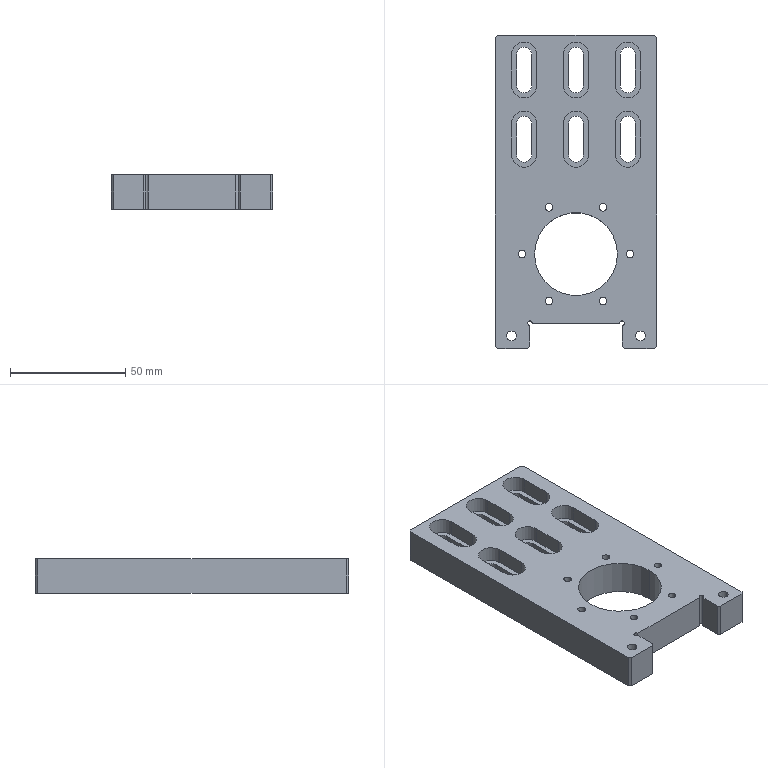Part | SolidWorks | features BaseBody 1 | 1 solid | 91 faces | box 70 x 136 x 15 mm | volume 103705 mm3 | plane 46 | cylinder 45 | commonest cylinder face diameters 3.3 x12 6.6 x12 11 x12 4.2 x4 2 x3 36 x2